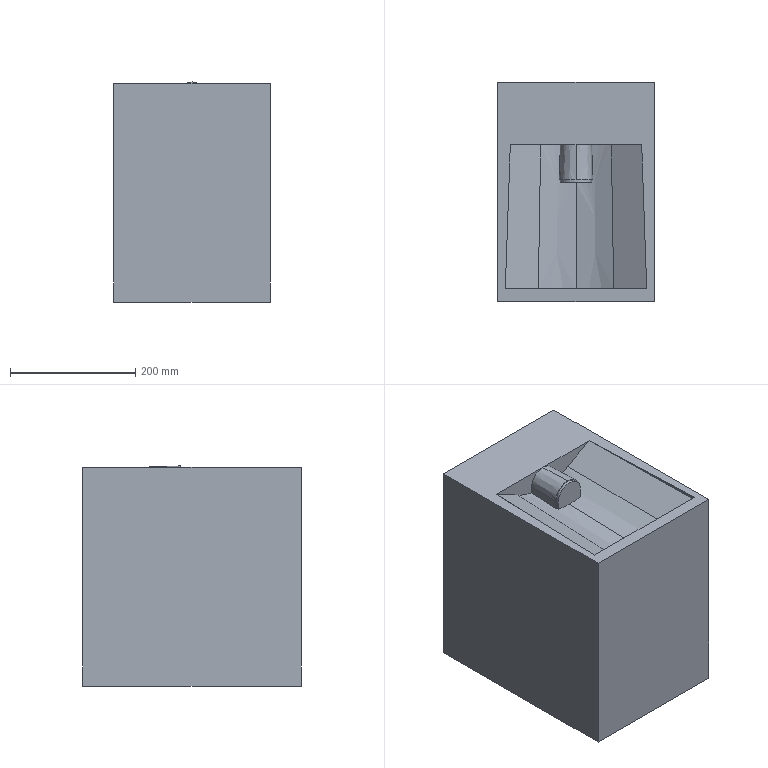Part | STEP file | Ice maker V1.201001 | 1 solid | 24 faces | box 250 x 350 x 351.956 mm | volume 29308107 mm3 | plane 19 | cone 5